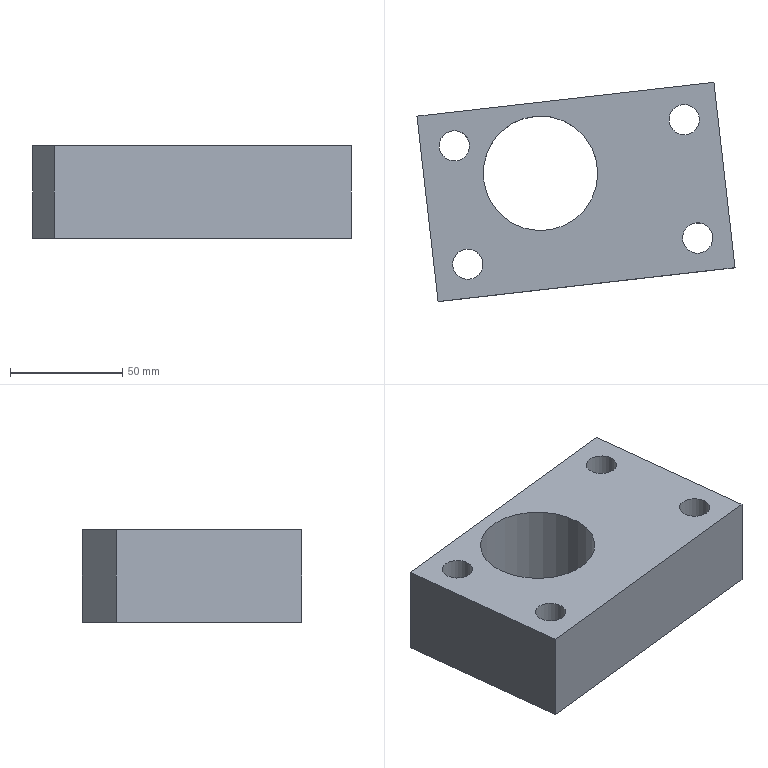Part | NX | features solid 2 | 1 solid | 19 faces | box 141.541 x 97.522 x 41 mm | volume 335107 mm3 | plane 10 | cylinder 9 | commonest cylinder face diameters 13.5 x4 20 x4 51 x1
STEP:
#1=CARTESIAN_POINT('',(2413.748,103.871,101.));
#2=VERTEX_POINT('',#1);
#3=CARTESIAN_POINT('',(2406.998,103.871,101.));
#4=DIRECTION('',(0.,0.,1.));
#5=DIRECTION('',(1.,0.,0.));
#6=AXIS2_PLACEMENT_3D('',#3,#4,#5);
#7=CIRCLE('',#6,6.75);
#8=EDGE_CURVE('',#2,#2,#7,.T.);
#9=ORIENTED_EDGE('',*,*,#8,.F.);
#10=EDGE_LOOP('',(#9));
#11=FACE_BOUND('',#10,.T.);
#12=CARTESIAN_POINT('',(2419.575,52.73,101.));
#13=VERTEX_POINT('',#12);
#14=CARTESIAN_POINT('',(2412.998,51.211,101.));
#15=DIRECTION('',(0.,0.,-1.));
#16=DIRECTION('',(0.9744,0.225,0.));
#17=AXIS2_PLACEMENT_3D('',#14,#15,#16);
#18=CIRCLE('',#17,6.75);
#19=EDGE_CURVE('',#13,#13,#18,.T.);
#20=ORIENTED_EDGE('',*,*,#19,.T.);
#21=EDGE_LOOP('',(#20));
#22=FACE_BOUND('',#21,.T.);
#23=CARTESIAN_POINT('',(2420.203,120.472,101.));
#24=VERTEX_POINT('',#23);
#25=CARTESIAN_POINT('',(2288.058,105.416,101.));
#26=VERTEX_POINT('',#25);
#27=CARTESIAN_POINT('',(2343.698,111.756,101.));
#28=DIRECTION('',(-0.9936,-0.1132,0.));
#29=VECTOR('',#28,1000.);
#30=LINE('',#27,#29);
#31=EDGE_CURVE('',#24,#26,#30,.T.);
#32=ORIENTED_EDGE('',*,*,#31,.T.);
#33=CARTESIAN_POINT('',(2297.454,22.95,101.));
#34=VERTEX_POINT('',#33);
#35=CARTESIAN_POINT('',(2292.36,67.661,101.));
#36=DIRECTION('',(0.1132,-0.9936,0.));
#37=VECTOR('',#36,1000.);
#38=LINE('',#35,#37);
#39=EDGE_CURVE('',#26,#34,#38,.T.);
#40=ORIENTED_EDGE('',*,*,#39,.T.);
#41=CARTESIAN_POINT('',(2429.599,38.006,101.));
#42=VERTEX_POINT('',#41);
#43=CARTESIAN_POINT('',(2353.094,29.289,101.));
#44=DIRECTION('',(0.9936,0.1132,0.));
#45=VECTOR('',#44,1000.);
#46=LINE('',#43,#45);
#47=EDGE_CURVE('',#34,#42,#46,.T.);
#48=ORIENTED_EDGE('',*,*,#47,.T.);
#49=CARTESIAN_POINT('',(2424.505,82.717,101.));
#50=DIRECTION('',(-0.1132,0.9936,0.));
#51=VECTOR('',#50,1000.);
#52=LINE('',#49,#51);
#53=EDGE_CURVE('',#42,#24,#52,.T.);
#54=ORIENTED_EDGE('',*,*,#53,.T.);
#55=EDGE_LOOP('',(#32,#40,#48,#54));
#56=FACE_BOUND('',#55,.T.);
#57=CARTESIAN_POINT('',(2368.5,80.,101.));
#58=VERTEX_POINT('',#57);
#59=CARTESIAN_POINT('',(2343.,80.,101.));
#60=DIRECTION('',(0.,0.,-1.));
#61=DIRECTION('',(1.,0.,0.));
#62=AXIS2_PLACEMENT_3D('',#59,#60,#61);
#63=CIRCLE('',#62,25.5);
#64=EDGE_CURVE('',#58,#58,#63,.T.);
#65=ORIENTED_EDGE('',*,*,#64,.T.);
#66=EDGE_LOOP('',(#65));
#67=FACE_BOUND('',#66,.T.);
#68=CARTESIAN_POINT('',(2298.083,90.692,101.));
#69=VERTEX_POINT('',#68);
#70=CARTESIAN_POINT('',(2304.66,92.211,101.));
#71=DIRECTION('',(0.,0.,-1.));
#72=DIRECTION('',(-0.9744,-0.225,0.));
#73=AXIS2_PLACEMENT_3D('',#70,#71,#72);
#74=CIRCLE('',#73,6.75);
#75=EDGE_CURVE('',#69,#69,#74,.T.);
#76=ORIENTED_EDGE('',*,*,#75,.T.);
#77=EDGE_LOOP('',(#76));
#78=FACE_BOUND('',#77,.T.);
#79=CARTESIAN_POINT('',(2303.91,39.552,101.));
#80=VERTEX_POINT('',#79);
#81=CARTESIAN_POINT('',(2310.66,39.552,101.));
#82=DIRECTION('',(0.,0.,1.));
#83=DIRECTION('',(-1.,0.,0.));
#84=AXIS2_PLACEMENT_3D('',#81,#82,#83);
#85=CIRCLE('',#84,6.75);
#86=EDGE_CURVE('',#80,#80,#85,.T.);
#87=ORIENTED_EDGE('',*,*,#86,.F.);
#88=EDGE_LOOP('',(#87));
#89=FACE_BOUND('',#88,.T.);
#90=CARTESIAN_POINT('',(94.5,-193.,101.));
#91=DIRECTION('',(0.,0.,1.));
#92=DIRECTION('',(-1.,0.,0.));
#93=AXIS2_PLACEMENT_3D('',#90,#91,#92);
#94=PLANE('',#93);
#95=ADVANCED_FACE('',(#11,#22,#56,#67,#78,#89),#94,.T.);
#96=CARTESIAN_POINT('',(2416.998,103.871,60.));
#97=VERTEX_POINT('',#96);
#98=CARTESIAN_POINT('',(2406.998,103.871,60.));
#99=DIRECTION('',(0.,0.,-1.));
#100=DIRECTION('',(1.,0.,0.));
#101=AXIS2_PLACEMENT_3D('',#98,#99,#100);
#102=CIRCLE('',#101,10.);
#103=EDGE_CURVE('',#97,#97,#102,.T.);
#104=ORIENTED_EDGE('',*,*,#103,.F.);
#105=EDGE_LOOP('',(#104));
#106=FACE_BOUND('',#105,.T.);
#107=CARTESIAN_POINT('',(2422.741,53.461,60.));
#108=VERTEX_POINT('',#107);
#109=CARTESIAN_POINT('',(2412.998,51.211,60.));
#110=DIRECTION('',(0.,0.,1.));
#111=DIRECTION('',(0.9744,0.225,0.));
#112=AXIS2_PLACEMENT_3D('',#109,#110,#111);
#113=CIRCLE('',#112,10.);
#114=EDGE_CURVE('',#108,#108,#113,.T.);
#115=ORIENTED_EDGE('',*,*,#114,.T.);
#116=EDGE_LOOP('',(#115));
#117=FACE_BOUND('',#116,.T.);
#118=CARTESIAN_POINT('',(2420.203,120.472,60.));
#119=VERTEX_POINT('',#118);
#120=CARTESIAN_POINT('',(2429.599,38.006,60.));
#121=VERTEX_POINT('',#120);
#122=CARTESIAN_POINT('',(2424.505,82.717,60.));
#123=DIRECTION('',(0.1132,-0.9936,0.));
#124=VECTOR('',#123,1000.);
#125=LINE('',#122,#124);
#126=EDGE_CURVE('',#119,#121,#125,.T.);
#127=ORIENTED_EDGE('',*,*,#126,.T.);
#128=CARTESIAN_POINT('',(2297.454,22.95,60.));
#129=VERTEX_POINT('',#128);
#130=CARTESIAN_POINT('',(2353.094,29.289,60.));
#131=DIRECTION('',(-0.9936,-0.1132,0.));
#132=VECTOR('',#131,1000.);
#133=LINE('',#130,#132);
#134=EDGE_CURVE('',#121,#129,#133,.T.);
#135=ORIENTED_EDGE('',*,*,#134,.T.);
#136=CARTESIAN_POINT('',(2288.058,105.416,60.));
#137=VERTEX_POINT('',#136);
#138=CARTESIAN_POINT('',(2292.36,67.661,60.));
#139=DIRECTION('',(-0.1132,0.9936,0.));
#140=VECTOR('',#139,1000.);
#141=LINE('',#138,#140);
#142=EDGE_CURVE('',#129,#137,#141,.T.);
#143=ORIENTED_EDGE('',*,*,#142,.T.);
#144=CARTESIAN_POINT('',(2343.698,111.756,60.));
#145=DIRECTION('',(0.9936,0.1132,0.));
#146=VECTOR('',#145,1000.);
#147=LINE('',#144,#146);
#148=EDGE_CURVE('',#137,#119,#147,.T.);
#149=ORIENTED_EDGE('',*,*,#148,.T.);
#150=EDGE_LOOP('',(#127,#135,#143,#149));
#151=FACE_BOUND('',#150,.T.);
#152=CARTESIAN_POINT('',(2368.5,80.,60.));
#153=VERTEX_POINT('',#152);
#154=CARTESIAN_POINT('',(2343.,80.,60.));
#155=DIRECTION('',(0.,0.,1.));
#156=DIRECTION('',(1.,0.,0.));
#157=AXIS2_PLACEMENT_3D('',#154,#155,#156);
#158=CIRCLE('',#157,25.5);
#159=EDGE_CURVE('',#153,#153,#158,.T.);
#160=ORIENTED_EDGE('',*,*,#159,.T.);
#161=EDGE_LOOP('',(#160));
#162=FACE_BOUND('',#161,.T.);
#163=CARTESIAN_POINT('',(2294.916,89.961,60.));
#164=VERTEX_POINT('',#163);
#165=CARTESIAN_POINT('',(2304.66,92.211,60.));
#166=DIRECTION('',(0.,0.,1.));
#167=DIRECTION('',(-0.9744,-0.225,0.));
#168=AXIS2_PLACEMENT_3D('',#165,#166,#167);
#169=CIRCLE('',#168,10.);
#170=EDGE_CURVE('',#164,#164,#169,.T.);
#171=ORIENTED_EDGE('',*,*,#170,.T.);
#172=EDGE_LOOP('',(#171));
#173=FACE_BOUND('',#172,.T.);
#174=CARTESIAN_POINT('',(2300.66,39.552,60.));
#175=VERTEX_POINT('',#174);
#176=CARTESIAN_POINT('',(2310.66,39.552,60.));
#177=DIRECTION('',(0.,0.,-1.));
#178=DIRECTION('',(-1.,0.,0.));
#179=AXIS2_PLACEMENT_3D('',#176,#177,#178);
#180=CIRCLE('',#179,10.);
#181=EDGE_CURVE('',#175,#175,#180,.T.);
#182=ORIENTED_EDGE('',*,*,#181,.F.);
#183=EDGE_LOOP('',(#182));
#184=FACE_BOUND('',#183,.T.);
#185=CARTESIAN_POINT('',(2470.641,285.511,60.));
#186=DIRECTION('',(0.,0.,1.));
#187=DIRECTION('',(-1.,0.,0.));
#188=AXIS2_PLACEMENT_3D('',#185,#186,#187);
#189=PLANE('',#188);
#190=ADVANCED_FACE('',(#106,#117,#151,#162,#173,#184),#189,.F.);
#191=CARTESIAN_POINT('',(2420.203,120.472,-10.));
#192=DIRECTION('',(0.,0.,1.));
#193=VECTOR('',#192,1000.);
#194=LINE('',#191,#193);
#195=EDGE_CURVE('',#119,#24,#194,.T.);
#196=ORIENTED_EDGE('',*,*,#195,.F.);
#197=ORIENTED_EDGE('',*,*,#148,.F.);
#198=CARTESIAN_POINT('',(2288.058,105.416,-10.));
#199=DIRECTION('',(0.,0.,1.));
#200=VECTOR('',#199,1000.);
#201=LINE('',#198,#200);
#202=EDGE_CURVE('',#137,#26,#201,.T.);
#203=ORIENTED_EDGE('',*,*,#202,.T.);
#204=ORIENTED_EDGE('',*,*,#31,.F.);
#205=EDGE_LOOP('',(#196,#197,#203,#204));
#206=FACE_BOUND('',#205,.T.);
#207=CARTESIAN_POINT('',(2343.698,111.756,-10.));
#208=DIRECTION('',(-0.1132,0.9936,0.));
#209=DIRECTION('',(-0.9936,-0.1132,0.));
#210=AXIS2_PLACEMENT_3D('',#207,#208,#209);
#211=PLANE('',#210);
#212=ADVANCED_FACE('',(#206),#211,.T.);
#213=ORIENTED_EDGE('',*,*,#202,.F.);
#214=ORIENTED_EDGE('',*,*,#142,.F.);
#215=CARTESIAN_POINT('',(2297.454,22.95,-10.));
#216=DIRECTION('',(0.,0.,1.));
#217=VECTOR('',#216,1000.);
#218=LINE('',#215,#217);
#219=EDGE_CURVE('',#129,#34,#218,.T.);
#220=ORIENTED_EDGE('',*,*,#219,.T.);
#221=ORIENTED_EDGE('',*,*,#39,.F.);
#222=EDGE_LOOP('',(#213,#214,#220,#221));
#223=FACE_BOUND('',#222,.T.);
#224=CARTESIAN_POINT('',(2292.36,67.661,-10.));
#225=DIRECTION('',(-0.9936,-0.1132,0.));
#226=DIRECTION('',(0.1132,-0.9936,0.));
#227=AXIS2_PLACEMENT_3D('',#224,#225,#226);
#228=PLANE('',#227);
#229=ADVANCED_FACE('',(#223),#228,.T.);
#230=ORIENTED_EDGE('',*,*,#219,.F.);
#231=ORIENTED_EDGE('',*,*,#134,.F.);
#232=CARTESIAN_POINT('',(2429.599,38.006,-10.));
#233=DIRECTION('',(0.,0.,1.));
#234=VECTOR('',#233,1000.);
#235=LINE('',#232,#234);
#236=EDGE_CURVE('',#121,#42,#235,.T.);
#237=ORIENTED_EDGE('',*,*,#236,.T.);
#238=ORIENTED_EDGE('',*,*,#47,.F.);
#239=EDGE_LOOP('',(#230,#231,#237,#238));
#240=FACE_BOUND('',#239,.T.);
#241=CARTESIAN_POINT('',(2353.094,29.289,-10.));
#242=DIRECTION('',(0.1132,-0.9936,0.));
#243=DIRECTION('',(0.9936,0.1132,0.));
#244=AXIS2_PLACEMENT_3D('',#241,#242,#243);
#245=PLANE('',#244);
#246=ADVANCED_FACE('',(#240),#245,.T.);
#247=ORIENTED_EDGE('',*,*,#126,.F.);
#248=ORIENTED_EDGE('',*,*,#195,.T.);
#249=ORIENTED_EDGE('',*,*,#53,.F.);
#250=ORIENTED_EDGE('',*,*,#236,.F.);
#251=EDGE_LOOP('',(#247,#248,#249,#250));
#252=FACE_BOUND('',#251,.T.);
#253=CARTESIAN_POINT('',(2424.505,82.717,-10.));
#254=DIRECTION('',(0.9936,0.1132,0.));
#255=DIRECTION('',(-0.1132,0.9936,0.));
#256=AXIS2_PLACEMENT_3D('',#253,#254,#255);
#257=PLANE('',#256);
#258=ADVANCED_FACE('',(#252),#257,.T.);
#259=ORIENTED_EDGE('',*,*,#64,.F.);
#260=EDGE_LOOP('',(#259));
#261=FACE_BOUND('',#260,.T.);
#262=ORIENTED_EDGE('',*,*,#159,.F.);
#263=EDGE_LOOP('',(#262));
#264=FACE_BOUND('',#263,.T.);
#265=CARTESIAN_POINT('',(2343.,80.,-101.));
#266=DIRECTION('',(0.,0.,1.));
#267=DIRECTION('',(-1.,0.,0.));
#268=AXIS2_PLACEMENT_3D('',#265,#266,#267);
#269=CYLINDRICAL_SURFACE('',#268,25.5);
#270=ADVANCED_FACE('',(#261,#264),#269,.F.);
#271=CARTESIAN_POINT('',(2419.575,52.73,75.));
#272=VERTEX_POINT('',#271);
#273=CARTESIAN_POINT('',(2412.998,51.211,75.));
#274=DIRECTION('',(0.,0.,1.));
#275=DIRECTION('',(0.9744,0.225,0.));
#276=AXIS2_PLACEMENT_3D('',#273,#274,#275);
#277=CIRCLE('',#276,6.75);
#278=EDGE_CURVE('',#272,#272,#277,.T.);
#279=ORIENTED_EDGE('',*,*,#278,.F.);
#280=EDGE_LOOP('',(#279));
#281=FACE_BOUND('',#280,.T.);
#282=ORIENTED_EDGE('',*,*,#19,.F.);
#283=EDGE_LOOP('',(#282));
#284=FACE_BOUND('',#283,.T.);
#285=CARTESIAN_POINT('',(2412.998,51.211,60.));
#286=DIRECTION('',(0.,0.,1.));
#287=DIRECTION('',(-0.9744,-0.225,0.));
#288=AXIS2_PLACEMENT_3D('',#285,#286,#287);
#289=CYLINDRICAL_SURFACE('',#288,6.75);
#290=ADVANCED_FACE('',(#281,#284),#289,.F.);
#291=ORIENTED_EDGE('',*,*,#278,.T.);
#292=EDGE_LOOP('',(#291));
#293=FACE_BOUND('',#292,.T.);
#294=CARTESIAN_POINT('',(2422.741,53.461,75.));
#295=VERTEX_POINT('',#294);
#296=CARTESIAN_POINT('',(2412.998,51.211,75.));
#297=DIRECTION('',(0.,0.,1.));
#298=DIRECTION('',(0.9744,0.225,0.));
#299=AXIS2_PLACEMENT_3D('',#296,#297,#298);
#300=CIRCLE('',#299,10.);
#301=EDGE_CURVE('',#295,#295,#300,.T.);
#302=ORIENTED_EDGE('',*,*,#301,.F.);
#303=EDGE_LOOP('',(#302));
#304=FACE_BOUND('',#303,.T.);
#305=CARTESIAN_POINT('',(2412.998,51.211,75.));
#306=DIRECTION('',(0.,0.,1.));
#307=DIRECTION('',(-0.9744,-0.225,0.));
#308=AXIS2_PLACEMENT_3D('',#305,#306,#307);
#309=PLANE('',#308);
#310=ADVANCED_FACE('',(#293,#304),#309,.F.);
#311=ORIENTED_EDGE('',*,*,#301,.T.);
#312=EDGE_LOOP('',(#311));
#313=FACE_BOUND('',#312,.T.);
#314=ORIENTED_EDGE('',*,*,#114,.F.);
#315=EDGE_LOOP('',(#314));
#316=FACE_BOUND('',#315,.T.);
#317=CARTESIAN_POINT('',(2412.998,51.211,60.));
#318=DIRECTION('',(0.,0.,1.));
#319=DIRECTION('',(-0.9744,-0.225,0.));
#320=AXIS2_PLACEMENT_3D('',#317,#318,#319);
#321=CYLINDRICAL_SURFACE('',#320,10.);
#322=ADVANCED_FACE('',(#313,#316),#321,.F.);
#323=CARTESIAN_POINT('',(2413.748,103.871,75.));
#324=VERTEX_POINT('',#323);
#325=CARTESIAN_POINT('',(2406.998,103.871,75.));
#326=DIRECTION('',(0.,0.,-1.));
#327=DIRECTION('',(1.,0.,0.));
#328=AXIS2_PLACEMENT_3D('',#325,#326,#327);
#329=CIRCLE('',#328,6.75);
#330=EDGE_CURVE('',#324,#324,#329,.T.);
#331=ORIENTED_EDGE('',*,*,#330,.T.);
#332=EDGE_LOOP('',(#331));
#333=FACE_BOUND('',#332,.T.);
#334=ORIENTED_EDGE('',*,*,#8,.T.);
#335=EDGE_LOOP('',(#334));
#336=FACE_BOUND('',#335,.T.);
#337=CARTESIAN_POINT('',(2406.998,103.871,60.));
#338=DIRECTION('',(0.,0.,1.));
#339=DIRECTION('',(-1.,0.,0.));
#340=AXIS2_PLACEMENT_3D('',#337,#338,#339);
#341=CYLINDRICAL_SURFACE('',#340,6.75);
#342=ADVANCED_FACE('',(#333,#336),#341,.F.);
#343=ORIENTED_EDGE('',*,*,#330,.F.);
#344=EDGE_LOOP('',(#343));
#345=FACE_BOUND('',#344,.T.);
#346=CARTESIAN_POINT('',(2416.998,103.871,75.));
#347=VERTEX_POINT('',#346);
#348=CARTESIAN_POINT('',(2406.998,103.871,75.));
#349=DIRECTION('',(0.,0.,-1.));
#350=DIRECTION('',(1.,0.,0.));
#351=AXIS2_PLACEMENT_3D('',#348,#349,#350);
#352=CIRCLE('',#351,10.);
#353=EDGE_CURVE('',#347,#347,#352,.T.);
#354=ORIENTED_EDGE('',*,*,#353,.T.);
#355=EDGE_LOOP('',(#354));
#356=FACE_BOUND('',#355,.T.);
#357=CARTESIAN_POINT('',(2405.073,120.761,75.));
#358=DIRECTION('',(0.,0.,1.));
#359=DIRECTION('',(-1.,0.,0.));
#360=AXIS2_PLACEMENT_3D('',#357,#358,#359);
#361=PLANE('',#360);
#362=ADVANCED_FACE('',(#345,#356),#361,.F.);
#363=ORIENTED_EDGE('',*,*,#353,.F.);
#364=EDGE_LOOP('',(#363));
#365=FACE_BOUND('',#364,.T.);
#366=ORIENTED_EDGE('',*,*,#103,.T.);
#367=EDGE_LOOP('',(#366));
#368=FACE_BOUND('',#367,.T.);
#369=CARTESIAN_POINT('',(2406.998,103.871,60.));
#370=DIRECTION('',(0.,0.,1.));
#371=DIRECTION('',(-1.,0.,0.));
#372=AXIS2_PLACEMENT_3D('',#369,#370,#371);
#373=CYLINDRICAL_SURFACE('',#372,10.);
#374=ADVANCED_FACE('',(#365,#368),#373,.F.);
#375=CARTESIAN_POINT('',(2298.083,90.692,75.));
#376=VERTEX_POINT('',#375);
#377=CARTESIAN_POINT('',(2304.66,92.211,75.));
#378=DIRECTION('',(0.,0.,1.));
#379=DIRECTION('',(-0.9744,-0.225,0.));
#380=AXIS2_PLACEMENT_3D('',#377,#378,#379);
#381=CIRCLE('',#380,6.75);
#382=EDGE_CURVE('',#376,#376,#381,.T.);
#383=ORIENTED_EDGE('',*,*,#382,.F.);
#384=EDGE_LOOP('',(#383));
#385=FACE_BOUND('',#384,.T.);
#386=ORIENTED_EDGE('',*,*,#75,.F.);
#387=EDGE_LOOP('',(#386));
#388=FACE_BOUND('',#387,.T.);
#389=CARTESIAN_POINT('',(2304.66,92.211,60.));
#390=DIRECTION('',(0.,0.,1.));
#391=DIRECTION('',(0.9744,0.225,0.));
#392=AXIS2_PLACEMENT_3D('',#389,#390,#391);
#393=CYLINDRICAL_SURFACE('',#392,6.75);
#394=ADVANCED_FACE('',(#385,#388),#393,.F.);
#395=ORIENTED_EDGE('',*,*,#382,.T.);
#396=EDGE_LOOP('',(#395));
#397=FACE_BOUND('',#396,.T.);
#398=CARTESIAN_POINT('',(2294.916,89.961,75.));
#399=VERTEX_POINT('',#398);
#400=CARTESIAN_POINT('',(2304.66,92.211,75.));
#401=DIRECTION('',(0.,0.,1.));
#402=DIRECTION('',(-0.9744,-0.225,0.));
#403=AXIS2_PLACEMENT_3D('',#400,#401,#402);
#404=CIRCLE('',#403,10.);
#405=EDGE_CURVE('',#399,#399,#404,.T.);
#406=ORIENTED_EDGE('',*,*,#405,.F.);
#407=EDGE_LOOP('',(#406));
#408=FACE_BOUND('',#407,.T.);
#409=CARTESIAN_POINT('',(2302.735,109.102,75.));
#410=DIRECTION('',(0.,0.,1.));
#411=DIRECTION('',(0.9744,0.225,0.));
#412=AXIS2_PLACEMENT_3D('',#409,#410,#411);
#413=PLANE('',#412);
#414=ADVANCED_FACE('',(#397,#408),#413,.F.);
#415=ORIENTED_EDGE('',*,*,#405,.T.);
#416=EDGE_LOOP('',(#415));
#417=FACE_BOUND('',#416,.T.);
#418=ORIENTED_EDGE('',*,*,#170,.F.);
#419=EDGE_LOOP('',(#418));
#420=FACE_BOUND('',#419,.T.);
#421=CARTESIAN_POINT('',(2304.66,92.211,60.));
#422=DIRECTION('',(0.,0.,1.));
#423=DIRECTION('',(0.9744,0.225,0.));
#424=AXIS2_PLACEMENT_3D('',#421,#422,#423);
#425=CYLINDRICAL_SURFACE('',#424,10.);
#426=ADVANCED_FACE('',(#417,#420),#425,.F.);
#427=CARTESIAN_POINT('',(2303.91,39.552,75.));
#428=VERTEX_POINT('',#427);
#429=CARTESIAN_POINT('',(2310.66,39.552,75.));
#430=DIRECTION('',(0.,0.,-1.));
#431=DIRECTION('',(-1.,0.,0.));
#432=AXIS2_PLACEMENT_3D('',#429,#430,#431);
#433=CIRCLE('',#432,6.75);
#434=EDGE_CURVE('',#428,#428,#433,.T.);
#435=ORIENTED_EDGE('',*,*,#434,.T.);
#436=EDGE_LOOP('',(#435));
#437=FACE_BOUND('',#436,.T.);
#438=ORIENTED_EDGE('',*,*,#86,.T.);
#439=EDGE_LOOP('',(#438));
#440=FACE_BOUND('',#439,.T.);
#441=CARTESIAN_POINT('',(2310.66,39.552,60.));
#442=DIRECTION('',(0.,0.,1.));
#443=DIRECTION('',(1.,0.,0.));
#444=AXIS2_PLACEMENT_3D('',#441,#442,#443);
#445=CYLINDRICAL_SURFACE('',#444,6.75);
#446=ADVANCED_FACE('',(#437,#440),#445,.F.);
#447=ORIENTED_EDGE('',*,*,#434,.F.);
#448=EDGE_LOOP('',(#447));
#449=FACE_BOUND('',#448,.T.);
#450=CARTESIAN_POINT('',(2300.66,39.552,75.));
#451=VERTEX_POINT('',#450);
#452=CARTESIAN_POINT('',(2310.66,39.552,75.));
#453=DIRECTION('',(0.,0.,-1.));
#454=DIRECTION('',(-1.,0.,0.));
#455=AXIS2_PLACEMENT_3D('',#452,#453,#454);
#456=CIRCLE('',#455,10.);
#457=EDGE_CURVE('',#451,#451,#456,.T.);
#458=ORIENTED_EDGE('',*,*,#457,.T.);
#459=EDGE_LOOP('',(#458));
#460=FACE_BOUND('',#459,.T.);
#461=CARTESIAN_POINT('',(2310.66,39.552,75.));
#462=DIRECTION('',(0.,0.,1.));
#463=DIRECTION('',(1.,0.,0.));
#464=AXIS2_PLACEMENT_3D('',#461,#462,#463);
#465=PLANE('',#464);
#466=ADVANCED_FACE('',(#449,#460),#465,.F.);
#467=ORIENTED_EDGE('',*,*,#457,.F.);
#468=EDGE_LOOP('',(#467));
#469=FACE_BOUND('',#468,.T.);
#470=ORIENTED_EDGE('',*,*,#181,.T.);
#471=EDGE_LOOP('',(#470));
#472=FACE_BOUND('',#471,.T.);
#473=CARTESIAN_POINT('',(2310.66,39.552,60.));
#474=DIRECTION('',(0.,0.,1.));
#475=DIRECTION('',(1.,0.,0.));
#476=AXIS2_PLACEMENT_3D('',#473,#474,#475);
#477=CYLINDRICAL_SURFACE('',#476,10.);
#478=ADVANCED_FACE('',(#469,#472),#477,.F.);
#479=CLOSED_SHELL('',(#95,#190,#212,#229,#246,#258,#270,#290,#310,#322,#342,#362,#374,#394,#414,#426,#446,#466,#478));
#480=MANIFOLD_SOLID_BREP('',#479);
#481=(LENGTH_UNIT()NAMED_UNIT(*)SI_UNIT(.MILLI.,.METRE.));
#482=UNCERTAINTY_MEASURE_WITH_UNIT(LENGTH_MEASURE(0.00001),#481,'','');
#483=(NAMED_UNIT(*)PLANE_ANGLE_UNIT()SI_UNIT($,.RADIAN.));
#484=(NAMED_UNIT(*)SI_UNIT($,.STERADIAN.)SOLID_ANGLE_UNIT());
#485=(GEOMETRIC_REPRESENTATION_CONTEXT(3)GLOBAL_UNCERTAINTY_ASSIGNED_CONTEXT((#482))GLOBAL_UNIT_ASSIGNED_CONTEXT((#481,#483,#484))REPRESENTATION_CONTEXT('',''));
#486=ADVANCED_BREP_SHAPE_REPRESENTATION('',(#480),#485);